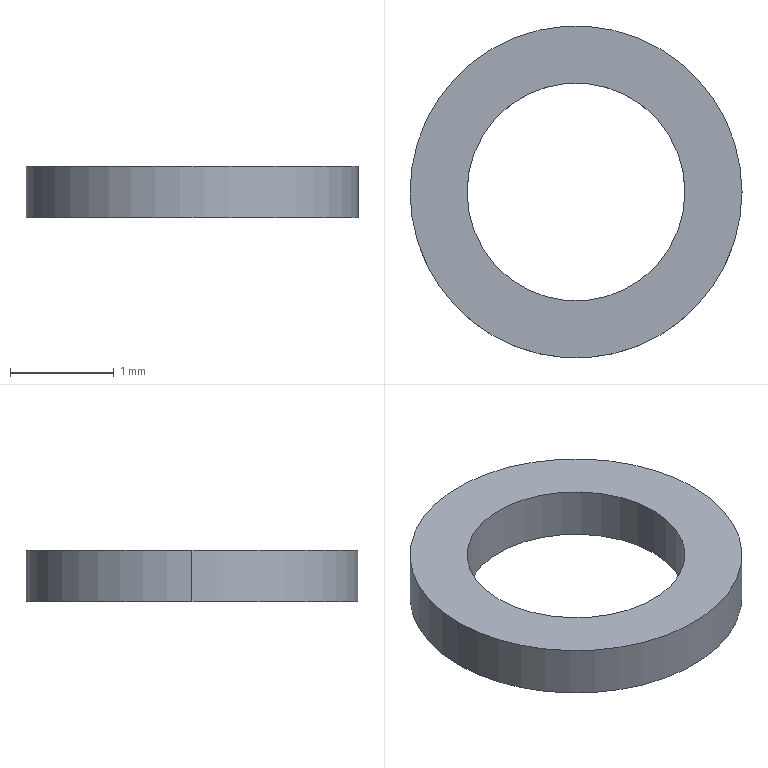Part | SolidWorks | features Extrusion 1 | 1 solid | 6 faces | box 3.2 x 3.2 x 0.5 mm | volume 2.289 mm3 | cylinder 4 | plane 2 | commonest cylinder face diameters 2.1 x2 3.2 x2
STEP:
#1=CARTESIAN_POINT('',(-1.05,0.,0.25));
#2=VERTEX_POINT('',#1);
#3=CARTESIAN_POINT('',(1.05,0.,0.25));
#4=VERTEX_POINT('',#3);
#5=CARTESIAN_POINT('',(0.,0.,0.25));
#6=DIRECTION('',(0.,0.,1.));
#7=DIRECTION('',(1.,0.,0.));
#8=AXIS2_PLACEMENT_3D('',#5,#6,#7);
#9=CIRCLE('',#8,1.05);
#10=EDGE_CURVE('',#2,#4,#9,.T.);
#11=ORIENTED_EDGE('',*,*,#10,.T.);
#12=CARTESIAN_POINT('',(1.05,0.,-0.25));
#13=VERTEX_POINT('',#12);
#14=CARTESIAN_POINT('',(1.05,0.,0.25));
#15=DIRECTION('',(0.,0.,-1.));
#16=VECTOR('',#15,1000.);
#17=LINE('',#14,#16);
#18=EDGE_CURVE('',#4,#13,#17,.T.);
#19=ORIENTED_EDGE('',*,*,#18,.T.);
#20=CARTESIAN_POINT('',(-1.05,0.,-0.25));
#21=VERTEX_POINT('',#20);
#22=CARTESIAN_POINT('',(0.,0.,-0.25));
#23=DIRECTION('',(0.,0.,1.));
#24=DIRECTION('',(1.,0.,0.));
#25=AXIS2_PLACEMENT_3D('',#22,#23,#24);
#26=CIRCLE('',#25,1.05);
#27=EDGE_CURVE('',#21,#13,#26,.T.);
#28=ORIENTED_EDGE('',*,*,#27,.F.);
#29=CARTESIAN_POINT('',(-1.05,0.,0.25));
#30=DIRECTION('',(0.,0.,-1.));
#31=VECTOR('',#30,1000.);
#32=LINE('',#29,#31);
#33=EDGE_CURVE('',#2,#21,#32,.T.);
#34=ORIENTED_EDGE('',*,*,#33,.F.);
#35=EDGE_LOOP('',(#11,#19,#28,#34));
#36=FACE_OUTER_BOUND('',#35,.T.);
#37=CARTESIAN_POINT('',(0.,0.,0.25));
#38=DIRECTION('',(0.,0.,-1.));
#39=DIRECTION('',(-1.,0.,0.));
#40=AXIS2_PLACEMENT_3D('',#37,#38,#39);
#41=CYLINDRICAL_SURFACE('',#40,1.05);
#42=ADVANCED_FACE('',(#36),#41,.F.);
#43=CARTESIAN_POINT('',(1.6,0.,0.25));
#44=VERTEX_POINT('',#43);
#45=CARTESIAN_POINT('',(-1.6,0.,0.25));
#46=VERTEX_POINT('',#45);
#47=CARTESIAN_POINT('',(0.,0.,0.25));
#48=DIRECTION('',(0.,0.,1.));
#49=DIRECTION('',(1.,0.,0.));
#50=AXIS2_PLACEMENT_3D('',#47,#48,#49);
#51=CIRCLE('',#50,1.6);
#52=EDGE_CURVE('',#44,#46,#51,.T.);
#53=ORIENTED_EDGE('',*,*,#52,.F.);
#54=CARTESIAN_POINT('',(1.6,0.,-0.25));
#55=VERTEX_POINT('',#54);
#56=CARTESIAN_POINT('',(1.6,0.,0.25));
#57=DIRECTION('',(0.,0.,-1.));
#58=VECTOR('',#57,1000.);
#59=LINE('',#56,#58);
#60=EDGE_CURVE('',#44,#55,#59,.T.);
#61=ORIENTED_EDGE('',*,*,#60,.T.);
#62=CARTESIAN_POINT('',(-1.6,0.,-0.25));
#63=VERTEX_POINT('',#62);
#64=CARTESIAN_POINT('',(0.,0.,-0.25));
#65=DIRECTION('',(0.,0.,1.));
#66=DIRECTION('',(1.,0.,0.));
#67=AXIS2_PLACEMENT_3D('',#64,#65,#66);
#68=CIRCLE('',#67,1.6);
#69=EDGE_CURVE('',#55,#63,#68,.T.);
#70=ORIENTED_EDGE('',*,*,#69,.T.);
#71=CARTESIAN_POINT('',(-1.6,0.,0.25));
#72=DIRECTION('',(0.,0.,-1.));
#73=VECTOR('',#72,1000.);
#74=LINE('',#71,#73);
#75=EDGE_CURVE('',#46,#63,#74,.T.);
#76=ORIENTED_EDGE('',*,*,#75,.F.);
#77=EDGE_LOOP('',(#53,#61,#70,#76));
#78=FACE_OUTER_BOUND('',#77,.T.);
#79=CARTESIAN_POINT('',(0.,0.,0.25));
#80=DIRECTION('',(0.,0.,-1.));
#81=DIRECTION('',(-1.,0.,0.));
#82=AXIS2_PLACEMENT_3D('',#79,#80,#81);
#83=CYLINDRICAL_SURFACE('',#82,1.6);
#84=ADVANCED_FACE('',(#78),#83,.T.);
#85=CARTESIAN_POINT('',(0.,0.,0.25));
#86=DIRECTION('',(0.,0.,1.));
#87=DIRECTION('',(1.,0.,0.));
#88=AXIS2_PLACEMENT_3D('',#85,#86,#87);
#89=CIRCLE('',#88,1.6);
#90=EDGE_CURVE('',#46,#44,#89,.T.);
#91=ORIENTED_EDGE('',*,*,#90,.T.);
#92=ORIENTED_EDGE('',*,*,#52,.T.);
#93=EDGE_LOOP('',(#91,#92));
#94=FACE_OUTER_BOUND('',#93,.T.);
#95=ORIENTED_EDGE('',*,*,#10,.F.);
#96=CARTESIAN_POINT('',(0.,0.,0.25));
#97=DIRECTION('',(0.,0.,1.));
#98=DIRECTION('',(1.,0.,0.));
#99=AXIS2_PLACEMENT_3D('',#96,#97,#98);
#100=CIRCLE('',#99,1.05);
#101=EDGE_CURVE('',#4,#2,#100,.T.);
#102=ORIENTED_EDGE('',*,*,#101,.F.);
#103=EDGE_LOOP('',(#95,#102));
#104=FACE_BOUND('',#103,.T.);
#105=CARTESIAN_POINT('',(0.,0.,0.25));
#106=DIRECTION('',(0.,0.,1.));
#107=DIRECTION('',(1.,0.,0.));
#108=AXIS2_PLACEMENT_3D('',#105,#106,#107);
#109=PLANE('',#108);
#110=ADVANCED_FACE('',(#94,#104),#109,.T.);
#111=CARTESIAN_POINT('',(0.,0.,-0.25));
#112=DIRECTION('',(0.,0.,1.));
#113=DIRECTION('',(1.,0.,0.));
#114=AXIS2_PLACEMENT_3D('',#111,#112,#113);
#115=CIRCLE('',#114,1.6);
#116=EDGE_CURVE('',#63,#55,#115,.T.);
#117=ORIENTED_EDGE('',*,*,#116,.F.);
#118=ORIENTED_EDGE('',*,*,#69,.F.);
#119=EDGE_LOOP('',(#117,#118));
#120=FACE_OUTER_BOUND('',#119,.T.);
#121=ORIENTED_EDGE('',*,*,#27,.T.);
#122=CARTESIAN_POINT('',(0.,0.,-0.25));
#123=DIRECTION('',(0.,0.,1.));
#124=DIRECTION('',(1.,0.,0.));
#125=AXIS2_PLACEMENT_3D('',#122,#123,#124);
#126=CIRCLE('',#125,1.05);
#127=EDGE_CURVE('',#13,#21,#126,.T.);
#128=ORIENTED_EDGE('',*,*,#127,.T.);
#129=EDGE_LOOP('',(#121,#128));
#130=FACE_BOUND('',#129,.T.);
#131=CARTESIAN_POINT('',(0.,0.,-0.25));
#132=DIRECTION('',(0.,0.,1.));
#133=DIRECTION('',(1.,0.,0.));
#134=AXIS2_PLACEMENT_3D('',#131,#132,#133);
#135=PLANE('',#134);
#136=ADVANCED_FACE('',(#120,#130),#135,.F.);
#137=ORIENTED_EDGE('',*,*,#60,.F.);
#138=ORIENTED_EDGE('',*,*,#90,.F.);
#139=ORIENTED_EDGE('',*,*,#75,.T.);
#140=ORIENTED_EDGE('',*,*,#116,.T.);
#141=EDGE_LOOP('',(#137,#138,#139,#140));
#142=FACE_OUTER_BOUND('',#141,.T.);
#143=CARTESIAN_POINT('',(0.,0.,0.25));
#144=DIRECTION('',(0.,0.,-1.));
#145=DIRECTION('',(-1.,0.,0.));
#146=AXIS2_PLACEMENT_3D('',#143,#144,#145);
#147=CYLINDRICAL_SURFACE('',#146,1.6);
#148=ADVANCED_FACE('',(#142),#147,.T.);
#149=ORIENTED_EDGE('',*,*,#18,.F.);
#150=ORIENTED_EDGE('',*,*,#101,.T.);
#151=ORIENTED_EDGE('',*,*,#33,.T.);
#152=ORIENTED_EDGE('',*,*,#127,.F.);
#153=EDGE_LOOP('',(#149,#150,#151,#152));
#154=FACE_OUTER_BOUND('',#153,.T.);
#155=CARTESIAN_POINT('',(0.,0.,0.25));
#156=DIRECTION('',(0.,0.,-1.));
#157=DIRECTION('',(-1.,0.,0.));
#158=AXIS2_PLACEMENT_3D('',#155,#156,#157);
#159=CYLINDRICAL_SURFACE('',#158,1.05);
#160=ADVANCED_FACE('',(#154),#159,.F.);
#161=CLOSED_SHELL('',(#42,#84,#110,#136,#148,#160));
#162=MANIFOLD_SOLID_BREP('',#161);
#163=CARTESIAN_POINT('',(0.,0.,0.));
#164=DIRECTION('',(0.,0.,1.));
#165=DIRECTION('',(1.,0.,0.));
#166=AXIS2_PLACEMENT_3D('',#163,#164,#165);
#167=(LENGTH_UNIT()NAMED_UNIT(*)SI_UNIT(.MILLI.,.METRE.));
#168=UNCERTAINTY_MEASURE_WITH_UNIT(LENGTH_MEASURE(0.00001),#167,'','');
#169=(NAMED_UNIT(*)PLANE_ANGLE_UNIT()SI_UNIT($,.RADIAN.));
#170=(NAMED_UNIT(*)SI_UNIT($,.STERADIAN.)SOLID_ANGLE_UNIT());
#171=(GEOMETRIC_REPRESENTATION_CONTEXT(3)GLOBAL_UNCERTAINTY_ASSIGNED_CONTEXT((#168))GLOBAL_UNIT_ASSIGNED_CONTEXT((#167,#169,#170))REPRESENTATION_CONTEXT('',''));
#172=ADVANCED_BREP_SHAPE_REPRESENTATION('',(#162,#166),#171);